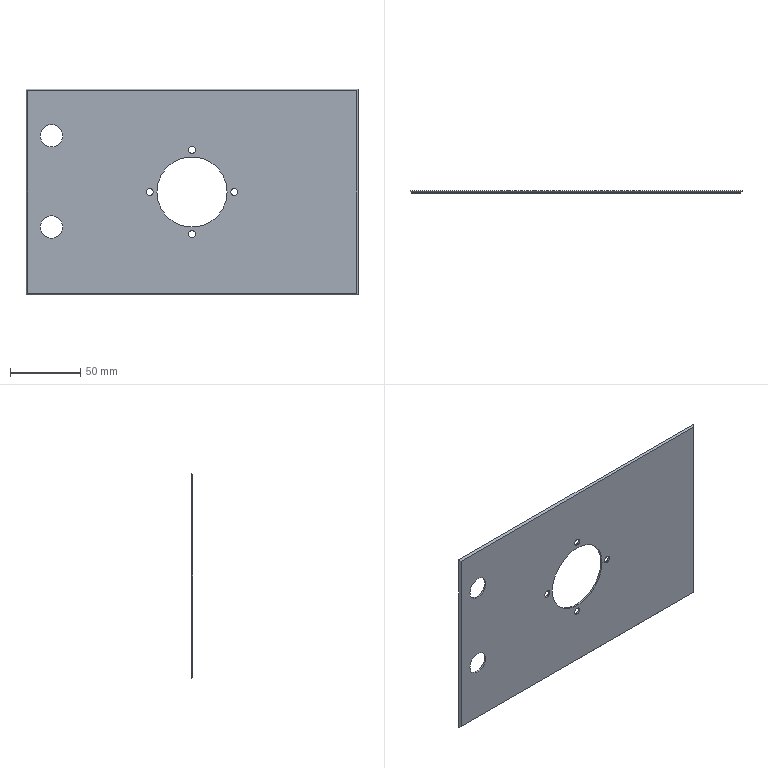Part | NX | 1 solid | 20 faces | box 236.4 x 1.2 x 146.4 mm | volume 38049 mm3 | cylinder 14 | plane 6 | commonest cylinder face diameters 5 x8 16 x4 50 x2
STEP:
#1=CARTESIAN_POINT('',(118.2,-108.8,73.2));
#2=VERTEX_POINT('',#1);
#3=CARTESIAN_POINT('',(118.2,-108.8,-73.2));
#4=VERTEX_POINT('',#3);
#5=CARTESIAN_POINT('',(118.2,-108.8,0.));
#6=DIRECTION('',(0.,0.,-1.));
#7=VECTOR('',#6,1000.);
#8=LINE('',#5,#7);
#9=EDGE_CURVE('',#2,#4,#8,.T.);
#10=ORIENTED_EDGE('',*,*,#9,.T.);
#11=CARTESIAN_POINT('',(-118.2,-108.8,-73.2));
#12=VERTEX_POINT('',#11);
#13=CARTESIAN_POINT('',(0.,-108.8,-73.2));
#14=DIRECTION('',(-1.,0.,0.));
#15=VECTOR('',#14,1000.);
#16=LINE('',#13,#15);
#17=EDGE_CURVE('',#4,#12,#16,.T.);
#18=ORIENTED_EDGE('',*,*,#17,.T.);
#19=CARTESIAN_POINT('',(-118.2,-108.8,73.2));
#20=VERTEX_POINT('',#19);
#21=CARTESIAN_POINT('',(-118.2,-108.8,0.));
#22=DIRECTION('',(0.,0.,-1.));
#23=VECTOR('',#22,1000.);
#24=LINE('',#21,#23);
#25=EDGE_CURVE('',#20,#12,#24,.T.);
#26=ORIENTED_EDGE('',*,*,#25,.F.);
#27=CARTESIAN_POINT('',(0.,-108.8,73.2));
#28=DIRECTION('',(-1.,0.,0.));
#29=VECTOR('',#28,1000.);
#30=LINE('',#27,#29);
#31=EDGE_CURVE('',#2,#20,#30,.T.);
#32=ORIENTED_EDGE('',*,*,#31,.F.);
#33=EDGE_LOOP('',(#10,#18,#26,#32));
#34=FACE_BOUND('',#33,.T.);
#35=CARTESIAN_POINT('',(-2.5,-108.8,-30.));
#36=VERTEX_POINT('',#35);
#37=CARTESIAN_POINT('',(2.5,-108.8,-30.));
#38=VERTEX_POINT('',#37);
#39=CARTESIAN_POINT('',(0.,-108.8,-30.));
#40=DIRECTION('',(0.,1.,0.));
#41=DIRECTION('',(1.,0.,0.));
#42=AXIS2_PLACEMENT_3D('',#39,#40,#41);
#43=CIRCLE('',#42,2.5);
#44=EDGE_CURVE('',#36,#38,#43,.T.);
#45=ORIENTED_EDGE('',*,*,#44,.F.);
#46=CARTESIAN_POINT('',(0.,-108.8,-30.));
#47=DIRECTION('',(0.,1.,0.));
#48=DIRECTION('',(1.,0.,0.));
#49=AXIS2_PLACEMENT_3D('',#46,#47,#48);
#50=CIRCLE('',#49,2.5);
#51=EDGE_CURVE('',#38,#36,#50,.T.);
#52=ORIENTED_EDGE('',*,*,#51,.F.);
#53=EDGE_LOOP('',(#45,#52));
#54=FACE_BOUND('',#53,.T.);
#55=CARTESIAN_POINT('',(32.5,-108.8,0.));
#56=VERTEX_POINT('',#55);
#57=CARTESIAN_POINT('',(27.5,-108.8,0.));
#58=VERTEX_POINT('',#57);
#59=CARTESIAN_POINT('',(30.,-108.8,0.));
#60=DIRECTION('',(0.,1.,0.));
#61=DIRECTION('',(1.,0.,0.));
#62=AXIS2_PLACEMENT_3D('',#59,#60,#61);
#63=CIRCLE('',#62,2.5);
#64=EDGE_CURVE('',#56,#58,#63,.T.);
#65=ORIENTED_EDGE('',*,*,#64,.F.);
#66=CARTESIAN_POINT('',(30.,-108.8,0.));
#67=DIRECTION('',(0.,1.,0.));
#68=DIRECTION('',(1.,0.,0.));
#69=AXIS2_PLACEMENT_3D('',#66,#67,#68);
#70=CIRCLE('',#69,2.5);
#71=EDGE_CURVE('',#58,#56,#70,.T.);
#72=ORIENTED_EDGE('',*,*,#71,.F.);
#73=EDGE_LOOP('',(#65,#72));
#74=FACE_BOUND('',#73,.T.);
#75=CARTESIAN_POINT('',(2.5,-108.8,30.));
#76=VERTEX_POINT('',#75);
#77=CARTESIAN_POINT('',(-2.5,-108.8,30.));
#78=VERTEX_POINT('',#77);
#79=CARTESIAN_POINT('',(0.,-108.8,30.));
#80=DIRECTION('',(0.,1.,0.));
#81=DIRECTION('',(1.,0.,0.));
#82=AXIS2_PLACEMENT_3D('',#79,#80,#81);
#83=CIRCLE('',#82,2.5);
#84=EDGE_CURVE('',#76,#78,#83,.T.);
#85=ORIENTED_EDGE('',*,*,#84,.F.);
#86=CARTESIAN_POINT('',(0.,-108.8,30.));
#87=DIRECTION('',(0.,1.,0.));
#88=DIRECTION('',(1.,0.,0.));
#89=AXIS2_PLACEMENT_3D('',#86,#87,#88);
#90=CIRCLE('',#89,2.5);
#91=EDGE_CURVE('',#78,#76,#90,.T.);
#92=ORIENTED_EDGE('',*,*,#91,.F.);
#93=EDGE_LOOP('',(#85,#92));
#94=FACE_BOUND('',#93,.T.);
#95=CARTESIAN_POINT('',(-32.5,-108.8,0.));
#96=VERTEX_POINT('',#95);
#97=CARTESIAN_POINT('',(-27.5,-108.8,0.));
#98=VERTEX_POINT('',#97);
#99=CARTESIAN_POINT('',(-30.,-108.8,0.));
#100=DIRECTION('',(0.,1.,0.));
#101=DIRECTION('',(1.,0.,0.));
#102=AXIS2_PLACEMENT_3D('',#99,#100,#101);
#103=CIRCLE('',#102,2.5);
#104=EDGE_CURVE('',#96,#98,#103,.T.);
#105=ORIENTED_EDGE('',*,*,#104,.F.);
#106=CARTESIAN_POINT('',(-30.,-108.8,0.));
#107=DIRECTION('',(0.,1.,0.));
#108=DIRECTION('',(1.,0.,0.));
#109=AXIS2_PLACEMENT_3D('',#106,#107,#108);
#110=CIRCLE('',#109,2.5);
#111=EDGE_CURVE('',#98,#96,#110,.T.);
#112=ORIENTED_EDGE('',*,*,#111,.F.);
#113=EDGE_LOOP('',(#105,#112));
#114=FACE_BOUND('',#113,.T.);
#115=CARTESIAN_POINT('',(-108.,-108.8,40.));
#116=VERTEX_POINT('',#115);
#117=CARTESIAN_POINT('',(-92.,-108.8,40.));
#118=VERTEX_POINT('',#117);
#119=CARTESIAN_POINT('',(-100.,-108.8,40.));
#120=DIRECTION('',(0.,-1.,0.));
#121=DIRECTION('',(1.,0.,0.));
#122=AXIS2_PLACEMENT_3D('',#119,#120,#121);
#123=CIRCLE('',#122,8.);
#124=EDGE_CURVE('',#116,#118,#123,.T.);
#125=ORIENTED_EDGE('',*,*,#124,.T.);
#126=CARTESIAN_POINT('',(-100.,-108.8,40.));
#127=DIRECTION('',(0.,-1.,0.));
#128=DIRECTION('',(1.,0.,0.));
#129=AXIS2_PLACEMENT_3D('',#126,#127,#128);
#130=CIRCLE('',#129,8.);
#131=EDGE_CURVE('',#118,#116,#130,.T.);
#132=ORIENTED_EDGE('',*,*,#131,.T.);
#133=EDGE_LOOP('',(#125,#132));
#134=FACE_BOUND('',#133,.T.);
#135=CARTESIAN_POINT('',(-108.,-108.8,-25.));
#136=VERTEX_POINT('',#135);
#137=CARTESIAN_POINT('',(-92.,-108.8,-25.));
#138=VERTEX_POINT('',#137);
#139=CARTESIAN_POINT('',(-100.,-108.8,-25.));
#140=DIRECTION('',(0.,1.,0.));
#141=DIRECTION('',(1.,0.,0.));
#142=AXIS2_PLACEMENT_3D('',#139,#140,#141);
#143=CIRCLE('',#142,8.);
#144=EDGE_CURVE('',#136,#138,#143,.T.);
#145=ORIENTED_EDGE('',*,*,#144,.F.);
#146=CARTESIAN_POINT('',(-100.,-108.8,-25.));
#147=DIRECTION('',(0.,1.,0.));
#148=DIRECTION('',(1.,0.,0.));
#149=AXIS2_PLACEMENT_3D('',#146,#147,#148);
#150=CIRCLE('',#149,8.);
#151=EDGE_CURVE('',#138,#136,#150,.T.);
#152=ORIENTED_EDGE('',*,*,#151,.F.);
#153=EDGE_LOOP('',(#145,#152));
#154=FACE_BOUND('',#153,.T.);
#155=CARTESIAN_POINT('',(25.,-108.8,0.));
#156=VERTEX_POINT('',#155);
#157=CARTESIAN_POINT('',(-25.,-108.8,0.));
#158=VERTEX_POINT('',#157);
#159=CARTESIAN_POINT('',(0.,-108.8,0.));
#160=DIRECTION('',(0.,1.,0.));
#161=DIRECTION('',(1.,0.,0.));
#162=AXIS2_PLACEMENT_3D('',#159,#160,#161);
#163=CIRCLE('',#162,25.);
#164=EDGE_CURVE('',#156,#158,#163,.T.);
#165=ORIENTED_EDGE('',*,*,#164,.F.);
#166=CARTESIAN_POINT('',(0.,-108.8,0.));
#167=DIRECTION('',(0.,1.,0.));
#168=DIRECTION('',(1.,0.,0.));
#169=AXIS2_PLACEMENT_3D('',#166,#167,#168);
#170=CIRCLE('',#169,25.);
#171=EDGE_CURVE('',#158,#156,#170,.T.);
#172=ORIENTED_EDGE('',*,*,#171,.F.);
#173=EDGE_LOOP('',(#165,#172));
#174=FACE_BOUND('',#173,.T.);
#175=CARTESIAN_POINT('',(-120.,-108.8,-75.));
#176=DIRECTION('',(0.,-1.,0.));
#177=DIRECTION('',(0.,0.,-1.));
#178=AXIS2_PLACEMENT_3D('',#175,#176,#177);
#179=PLANE('',#178);
#180=ADVANCED_FACE('',(#34,#54,#74,#94,#114,#134,#154,#174),#179,.F.);
#181=CARTESIAN_POINT('',(117.,-110.,72.));
#182=VERTEX_POINT('',#181);
#183=CARTESIAN_POINT('',(117.,-110.,-72.));
#184=VERTEX_POINT('',#183);
#185=CARTESIAN_POINT('',(117.,-110.,0.));
#186=DIRECTION('',(0.,0.,-1.));
#187=VECTOR('',#186,1000.);
#188=LINE('',#185,#187);
#189=EDGE_CURVE('',#182,#184,#188,.T.);
#190=ORIENTED_EDGE('',*,*,#189,.T.);
#191=CARTESIAN_POINT('',(45.,-182.,0.));
#192=DIRECTION('',(-0.5774,-0.5774,0.5774));
#193=VECTOR('',#192,1000.);
#194=LINE('',#191,#193);
#195=EDGE_CURVE('',#4,#184,#194,.T.);
#196=ORIENTED_EDGE('',*,*,#195,.F.);
#197=ORIENTED_EDGE('',*,*,#9,.F.);
#198=CARTESIAN_POINT('',(45.,-182.,0.));
#199=DIRECTION('',(-0.5774,-0.5774,-0.5774));
#200=VECTOR('',#199,1000.);
#201=LINE('',#198,#200);
#202=EDGE_CURVE('',#2,#182,#201,.T.);
#203=ORIENTED_EDGE('',*,*,#202,.T.);
#204=EDGE_LOOP('',(#190,#196,#197,#203));
#205=FACE_BOUND('',#204,.T.);
#206=CARTESIAN_POINT('',(118.5,-108.5,0.));
#207=DIRECTION('',(-0.7071,0.7071,0.));
#208=DIRECTION('',(0.,0.,1.));
#209=AXIS2_PLACEMENT_3D('',#206,#207,#208);
#210=PLANE('',#209);
#211=ADVANCED_FACE('',(#205),#210,.F.);
#212=CARTESIAN_POINT('',(-117.,-110.,72.));
#213=VERTEX_POINT('',#212);
#214=CARTESIAN_POINT('',(0.,-110.,72.));
#215=DIRECTION('',(-1.,0.,0.));
#216=VECTOR('',#215,1000.);
#217=LINE('',#214,#216);
#218=EDGE_CURVE('',#182,#213,#217,.T.);
#219=ORIENTED_EDGE('',*,*,#218,.F.);
#220=ORIENTED_EDGE('',*,*,#202,.F.);
#221=ORIENTED_EDGE('',*,*,#31,.T.);
#222=CARTESIAN_POINT('',(-45.,-182.,0.));
#223=DIRECTION('',(0.5774,-0.5774,-0.5774));
#224=VECTOR('',#223,1000.);
#225=LINE('',#222,#224);
#226=EDGE_CURVE('',#20,#213,#225,.T.);
#227=ORIENTED_EDGE('',*,*,#226,.T.);
#228=EDGE_LOOP('',(#219,#220,#221,#227));
#229=FACE_BOUND('',#228,.T.);
#230=CARTESIAN_POINT('',(0.,-108.5,73.5));
#231=DIRECTION('',(0.,-0.7071,0.7071));
#232=DIRECTION('',(-1.,0.,0.));
#233=AXIS2_PLACEMENT_3D('',#230,#231,#232);
#234=PLANE('',#233);
#235=ADVANCED_FACE('',(#229),#234,.T.);
#236=CARTESIAN_POINT('',(-117.,-110.,-72.));
#237=VERTEX_POINT('',#236);
#238=CARTESIAN_POINT('',(-117.,-110.,0.));
#239=DIRECTION('',(0.,0.,-1.));
#240=VECTOR('',#239,1000.);
#241=LINE('',#238,#240);
#242=EDGE_CURVE('',#213,#237,#241,.T.);
#243=ORIENTED_EDGE('',*,*,#242,.F.);
#244=ORIENTED_EDGE('',*,*,#226,.F.);
#245=ORIENTED_EDGE('',*,*,#25,.T.);
#246=CARTESIAN_POINT('',(-45.,-182.,0.));
#247=DIRECTION('',(0.5774,-0.5774,0.5774));
#248=VECTOR('',#247,1000.);
#249=LINE('',#246,#248);
#250=EDGE_CURVE('',#12,#237,#249,.T.);
#251=ORIENTED_EDGE('',*,*,#250,.T.);
#252=EDGE_LOOP('',(#243,#244,#245,#251));
#253=FACE_BOUND('',#252,.T.);
#254=CARTESIAN_POINT('',(-118.5,-108.5,0.));
#255=DIRECTION('',(-0.7071,-0.7071,0.));
#256=DIRECTION('',(-0.7071,0.7071,0.));
#257=AXIS2_PLACEMENT_3D('',#254,#255,#256);
#258=PLANE('',#257);
#259=ADVANCED_FACE('',(#253),#258,.T.);
#260=CARTESIAN_POINT('',(0.,-110.,-72.));
#261=DIRECTION('',(-1.,0.,0.));
#262=VECTOR('',#261,1000.);
#263=LINE('',#260,#262);
#264=EDGE_CURVE('',#184,#237,#263,.T.);
#265=ORIENTED_EDGE('',*,*,#264,.T.);
#266=ORIENTED_EDGE('',*,*,#250,.F.);
#267=ORIENTED_EDGE('',*,*,#17,.F.);
#268=ORIENTED_EDGE('',*,*,#195,.T.);
#269=EDGE_LOOP('',(#265,#266,#267,#268));
#270=FACE_BOUND('',#269,.T.);
#271=CARTESIAN_POINT('',(0.,-108.5,-73.5));
#272=DIRECTION('',(0.,0.7071,0.7071));
#273=DIRECTION('',(1.,0.,0.));
#274=AXIS2_PLACEMENT_3D('',#271,#272,#273);
#275=PLANE('',#274);
#276=ADVANCED_FACE('',(#270),#275,.F.);
#277=ORIENTED_EDGE('',*,*,#242,.T.);
#278=ORIENTED_EDGE('',*,*,#264,.F.);
#279=ORIENTED_EDGE('',*,*,#189,.F.);
#280=ORIENTED_EDGE('',*,*,#218,.T.);
#281=EDGE_LOOP('',(#277,#278,#279,#280));
#282=FACE_BOUND('',#281,.T.);
#283=CARTESIAN_POINT('',(27.5,-110.,0.));
#284=VERTEX_POINT('',#283);
#285=CARTESIAN_POINT('',(32.5,-110.,0.));
#286=VERTEX_POINT('',#285);
#287=CARTESIAN_POINT('',(30.,-110.,0.));
#288=DIRECTION('',(0.,-1.,0.));
#289=DIRECTION('',(-1.,0.,0.));
#290=AXIS2_PLACEMENT_3D('',#287,#288,#289);
#291=CIRCLE('',#290,2.5);
#292=EDGE_CURVE('',#284,#286,#291,.T.);
#293=ORIENTED_EDGE('',*,*,#292,.F.);
#294=CARTESIAN_POINT('',(30.,-110.,0.));
#295=DIRECTION('',(0.,-1.,0.));
#296=DIRECTION('',(-1.,0.,0.));
#297=AXIS2_PLACEMENT_3D('',#294,#295,#296);
#298=CIRCLE('',#297,2.5);
#299=EDGE_CURVE('',#286,#284,#298,.T.);
#300=ORIENTED_EDGE('',*,*,#299,.F.);
#301=EDGE_LOOP('',(#293,#300));
#302=FACE_BOUND('',#301,.T.);
#303=CARTESIAN_POINT('',(-2.5,-110.,30.));
#304=VERTEX_POINT('',#303);
#305=CARTESIAN_POINT('',(2.5,-110.,30.));
#306=VERTEX_POINT('',#305);
#307=CARTESIAN_POINT('',(0.,-110.,30.));
#308=DIRECTION('',(0.,-1.,0.));
#309=DIRECTION('',(-1.,0.,0.));
#310=AXIS2_PLACEMENT_3D('',#307,#308,#309);
#311=CIRCLE('',#310,2.5);
#312=EDGE_CURVE('',#304,#306,#311,.T.);
#313=ORIENTED_EDGE('',*,*,#312,.F.);
#314=CARTESIAN_POINT('',(0.,-110.,30.));
#315=DIRECTION('',(0.,-1.,0.));
#316=DIRECTION('',(-1.,0.,0.));
#317=AXIS2_PLACEMENT_3D('',#314,#315,#316);
#318=CIRCLE('',#317,2.5);
#319=EDGE_CURVE('',#306,#304,#318,.T.);
#320=ORIENTED_EDGE('',*,*,#319,.F.);
#321=EDGE_LOOP('',(#313,#320));
#322=FACE_BOUND('',#321,.T.);
#323=CARTESIAN_POINT('',(-32.5,-110.,0.));
#324=VERTEX_POINT('',#323);
#325=CARTESIAN_POINT('',(-27.5,-110.,0.));
#326=VERTEX_POINT('',#325);
#327=CARTESIAN_POINT('',(-30.,-110.,0.));
#328=DIRECTION('',(0.,-1.,0.));
#329=DIRECTION('',(-1.,0.,0.));
#330=AXIS2_PLACEMENT_3D('',#327,#328,#329);
#331=CIRCLE('',#330,2.5);
#332=EDGE_CURVE('',#324,#326,#331,.T.);
#333=ORIENTED_EDGE('',*,*,#332,.F.);
#334=CARTESIAN_POINT('',(-30.,-110.,0.));
#335=DIRECTION('',(0.,-1.,0.));
#336=DIRECTION('',(-1.,0.,0.));
#337=AXIS2_PLACEMENT_3D('',#334,#335,#336);
#338=CIRCLE('',#337,2.5);
#339=EDGE_CURVE('',#326,#324,#338,.T.);
#340=ORIENTED_EDGE('',*,*,#339,.F.);
#341=EDGE_LOOP('',(#333,#340));
#342=FACE_BOUND('',#341,.T.);
#343=CARTESIAN_POINT('',(-108.,-110.,40.));
#344=VERTEX_POINT('',#343);
#345=CARTESIAN_POINT('',(-92.,-110.,40.));
#346=VERTEX_POINT('',#345);
#347=CARTESIAN_POINT('',(-100.,-110.,40.));
#348=DIRECTION('',(0.,-1.,0.));
#349=DIRECTION('',(1.,0.,0.));
#350=AXIS2_PLACEMENT_3D('',#347,#348,#349);
#351=CIRCLE('',#350,8.);
#352=EDGE_CURVE('',#344,#346,#351,.T.);
#353=ORIENTED_EDGE('',*,*,#352,.F.);
#354=CARTESIAN_POINT('',(-100.,-110.,40.));
#355=DIRECTION('',(0.,-1.,0.));
#356=DIRECTION('',(1.,0.,0.));
#357=AXIS2_PLACEMENT_3D('',#354,#355,#356);
#358=CIRCLE('',#357,8.);
#359=EDGE_CURVE('',#346,#344,#358,.T.);
#360=ORIENTED_EDGE('',*,*,#359,.F.);
#361=EDGE_LOOP('',(#353,#360));
#362=FACE_BOUND('',#361,.T.);
#363=CARTESIAN_POINT('',(-108.,-110.,-25.));
#364=VERTEX_POINT('',#363);
#365=CARTESIAN_POINT('',(-92.,-110.,-25.));
#366=VERTEX_POINT('',#365);
#367=CARTESIAN_POINT('',(-100.,-110.,-25.));
#368=DIRECTION('',(0.,-1.,0.));
#369=DIRECTION('',(-1.,0.,0.));
#370=AXIS2_PLACEMENT_3D('',#367,#368,#369);
#371=CIRCLE('',#370,8.);
#372=EDGE_CURVE('',#364,#366,#371,.T.);
#373=ORIENTED_EDGE('',*,*,#372,.F.);
#374=CARTESIAN_POINT('',(-100.,-110.,-25.));
#375=DIRECTION('',(0.,-1.,0.));
#376=DIRECTION('',(-1.,0.,0.));
#377=AXIS2_PLACEMENT_3D('',#374,#375,#376);
#378=CIRCLE('',#377,8.);
#379=EDGE_CURVE('',#366,#364,#378,.T.);
#380=ORIENTED_EDGE('',*,*,#379,.F.);
#381=EDGE_LOOP('',(#373,#380));
#382=FACE_BOUND('',#381,.T.);
#383=CARTESIAN_POINT('',(25.,-110.,0.));
#384=VERTEX_POINT('',#383);
#385=CARTESIAN_POINT('',(-25.,-110.,0.));
#386=VERTEX_POINT('',#385);
#387=CARTESIAN_POINT('',(0.,-110.,0.));
#388=DIRECTION('',(0.,-1.,0.));
#389=DIRECTION('',(-1.,0.,0.));
#390=AXIS2_PLACEMENT_3D('',#387,#388,#389);
#391=CIRCLE('',#390,25.);
#392=EDGE_CURVE('',#384,#386,#391,.T.);
#393=ORIENTED_EDGE('',*,*,#392,.F.);
#394=CARTESIAN_POINT('',(0.,-110.,0.));
#395=DIRECTION('',(0.,-1.,0.));
#396=DIRECTION('',(-1.,0.,0.));
#397=AXIS2_PLACEMENT_3D('',#394,#395,#396);
#398=CIRCLE('',#397,25.);
#399=EDGE_CURVE('',#386,#384,#398,.T.);
#400=ORIENTED_EDGE('',*,*,#399,.F.);
#401=EDGE_LOOP('',(#393,#400));
#402=FACE_BOUND('',#401,.T.);
#403=CARTESIAN_POINT('',(-2.5,-110.,-30.));
#404=VERTEX_POINT('',#403);
#405=CARTESIAN_POINT('',(2.5,-110.,-30.));
#406=VERTEX_POINT('',#405);
#407=CARTESIAN_POINT('',(0.,-110.,-30.));
#408=DIRECTION('',(0.,-1.,0.));
#409=DIRECTION('',(-1.,0.,0.));
#410=AXIS2_PLACEMENT_3D('',#407,#408,#409);
#411=CIRCLE('',#410,2.5);
#412=EDGE_CURVE('',#404,#406,#411,.T.);
#413=ORIENTED_EDGE('',*,*,#412,.F.);
#414=CARTESIAN_POINT('',(0.,-110.,-30.));
#415=DIRECTION('',(0.,-1.,0.));
#416=DIRECTION('',(-1.,0.,0.));
#417=AXIS2_PLACEMENT_3D('',#414,#415,#416);
#418=CIRCLE('',#417,2.5);
#419=EDGE_CURVE('',#406,#404,#418,.T.);
#420=ORIENTED_EDGE('',*,*,#419,.F.);
#421=EDGE_LOOP('',(#413,#420));
#422=FACE_BOUND('',#421,.T.);
#423=CARTESIAN_POINT('',(-120.,-110.,-75.));
#424=DIRECTION('',(0.,-1.,0.));
#425=DIRECTION('',(0.,0.,-1.));
#426=AXIS2_PLACEMENT_3D('',#423,#424,#425);
#427=PLANE('',#426);
#428=ADVANCED_FACE('',(#282,#302,#322,#342,#362,#382,#402,#422),#427,.T.);
#429=ORIENTED_EDGE('',*,*,#292,.T.);
#430=CARTESIAN_POINT('',(32.5,-110.,0.));
#431=DIRECTION('',(0.,1.,0.));
#432=VECTOR('',#431,1000.);
#433=LINE('',#430,#432);
#434=EDGE_CURVE('',#56,#286,#433,.F.);
#435=ORIENTED_EDGE('',*,*,#434,.F.);
#436=ORIENTED_EDGE('',*,*,#64,.T.);
#437=CARTESIAN_POINT('',(27.5,-110.,0.));
#438=DIRECTION('',(0.,1.,0.));
#439=VECTOR('',#438,1000.);
#440=LINE('',#437,#439);
#441=EDGE_CURVE('',#58,#284,#440,.F.);
#442=ORIENTED_EDGE('',*,*,#441,.T.);
#443=EDGE_LOOP('',(#429,#435,#436,#442));
#444=FACE_BOUND('',#443,.T.);
#445=CARTESIAN_POINT('',(30.,-110.,0.));
#446=DIRECTION('',(0.,1.,0.));
#447=DIRECTION('',(-1.,0.,0.));
#448=AXIS2_PLACEMENT_3D('',#445,#446,#447);
#449=CYLINDRICAL_SURFACE('',#448,2.5);
#450=ADVANCED_FACE('',(#444),#449,.F.);
#451=ORIENTED_EDGE('',*,*,#312,.T.);
#452=CARTESIAN_POINT('',(2.5,-110.,30.));
#453=DIRECTION('',(0.,1.,0.));
#454=VECTOR('',#453,1000.);
#455=LINE('',#452,#454);
#456=EDGE_CURVE('',#76,#306,#455,.F.);
#457=ORIENTED_EDGE('',*,*,#456,.F.);
#458=ORIENTED_EDGE('',*,*,#84,.T.);
#459=CARTESIAN_POINT('',(-2.5,-110.,30.));
#460=DIRECTION('',(0.,1.,0.));
#461=VECTOR('',#460,1000.);
#462=LINE('',#459,#461);
#463=EDGE_CURVE('',#78,#304,#462,.F.);
#464=ORIENTED_EDGE('',*,*,#463,.T.);
#465=EDGE_LOOP('',(#451,#457,#458,#464));
#466=FACE_BOUND('',#465,.T.);
#467=CARTESIAN_POINT('',(0.,-110.,30.));
#468=DIRECTION('',(0.,1.,0.));
#469=DIRECTION('',(-1.,0.,0.));
#470=AXIS2_PLACEMENT_3D('',#467,#468,#469);
#471=CYLINDRICAL_SURFACE('',#470,2.5);
#472=ADVANCED_FACE('',(#466),#471,.F.);
#473=ORIENTED_EDGE('',*,*,#104,.T.);
#474=CARTESIAN_POINT('',(-27.5,-110.,0.));
#475=DIRECTION('',(0.,1.,0.));
#476=VECTOR('',#475,1000.);
#477=LINE('',#474,#476);
#478=EDGE_CURVE('',#326,#98,#477,.T.);
#479=ORIENTED_EDGE('',*,*,#478,.F.);
#480=ORIENTED_EDGE('',*,*,#339,.T.);
#481=CARTESIAN_POINT('',(-32.5,-110.,0.));
#482=DIRECTION('',(0.,1.,0.));
#483=VECTOR('',#482,1000.);
#484=LINE('',#481,#483);
#485=EDGE_CURVE('',#324,#96,#484,.T.);
#486=ORIENTED_EDGE('',*,*,#485,.T.);
#487=EDGE_LOOP('',(#473,#479,#480,#486));
#488=FACE_BOUND('',#487,.T.);
#489=CARTESIAN_POINT('',(-30.,-110.,0.));
#490=DIRECTION('',(0.,1.,0.));
#491=DIRECTION('',(-1.,0.,0.));
#492=AXIS2_PLACEMENT_3D('',#489,#490,#491);
#493=CYLINDRICAL_SURFACE('',#492,2.5);
#494=ADVANCED_FACE('',(#488),#493,.F.);
#495=ORIENTED_EDGE('',*,*,#352,.T.);
#496=CARTESIAN_POINT('',(-92.,-110.,40.));
#497=DIRECTION('',(0.,-1.,0.));
#498=VECTOR('',#497,1000.);
#499=LINE('',#496,#498);
#500=EDGE_CURVE('',#118,#346,#499,.T.);
#501=ORIENTED_EDGE('',*,*,#500,.F.);
#502=ORIENTED_EDGE('',*,*,#124,.F.);
#503=CARTESIAN_POINT('',(-108.,-110.,40.));
#504=DIRECTION('',(0.,-1.,0.));
#505=VECTOR('',#504,1000.);
#506=LINE('',#503,#505);
#507=EDGE_CURVE('',#116,#344,#506,.T.);
#508=ORIENTED_EDGE('',*,*,#507,.T.);
#509=EDGE_LOOP('',(#495,#501,#502,#508));
#510=FACE_BOUND('',#509,.T.);
#511=CARTESIAN_POINT('',(-100.,-110.,40.));
#512=DIRECTION('',(0.,-1.,0.));
#513=DIRECTION('',(1.,0.,0.));
#514=AXIS2_PLACEMENT_3D('',#511,#512,#513);
#515=CYLINDRICAL_SURFACE('',#514,8.);
#516=ADVANCED_FACE('',(#510),#515,.F.);
#517=ORIENTED_EDGE('',*,*,#144,.T.);
#518=CARTESIAN_POINT('',(-92.,-110.,-25.));
#519=DIRECTION('',(0.,1.,0.));
#520=VECTOR('',#519,1000.);
#521=LINE('',#518,#520);
#522=EDGE_CURVE('',#366,#138,#521,.T.);
#523=ORIENTED_EDGE('',*,*,#522,.F.);
#524=ORIENTED_EDGE('',*,*,#379,.T.);
#525=CARTESIAN_POINT('',(-108.,-110.,-25.));
#526=DIRECTION('',(0.,1.,0.));
#527=VECTOR('',#526,1000.);
#528=LINE('',#525,#527);
#529=EDGE_CURVE('',#364,#136,#528,.T.);
#530=ORIENTED_EDGE('',*,*,#529,.T.);
#531=EDGE_LOOP('',(#517,#523,#524,#530));
#532=FACE_BOUND('',#531,.T.);
#533=CARTESIAN_POINT('',(-100.,-110.,-25.));
#534=DIRECTION('',(0.,1.,0.));
#535=DIRECTION('',(-1.,0.,0.));
#536=AXIS2_PLACEMENT_3D('',#533,#534,#535);
#537=CYLINDRICAL_SURFACE('',#536,8.);
#538=ADVANCED_FACE('',(#532),#537,.F.);
#539=ORIENTED_EDGE('',*,*,#392,.T.);
#540=CARTESIAN_POINT('',(-25.,-110.,0.));
#541=DIRECTION('',(0.,1.,0.));
#542=VECTOR('',#541,1000.);
#543=LINE('',#540,#542);
#544=EDGE_CURVE('',#158,#386,#543,.F.);
#545=ORIENTED_EDGE('',*,*,#544,.F.);
#546=ORIENTED_EDGE('',*,*,#171,.T.);
#547=CARTESIAN_POINT('',(25.,-110.,0.));
#548=DIRECTION('',(0.,1.,0.));
#549=VECTOR('',#548,1000.);
#550=LINE('',#547,#549);
#551=EDGE_CURVE('',#156,#384,#550,.F.);
#552=ORIENTED_EDGE('',*,*,#551,.T.);
#553=EDGE_LOOP('',(#539,#545,#546,#552));
#554=FACE_BOUND('',#553,.T.);
#555=CARTESIAN_POINT('',(0.,-110.,0.));
#556=DIRECTION('',(0.,1.,0.));
#557=DIRECTION('',(-1.,0.,0.));
#558=AXIS2_PLACEMENT_3D('',#555,#556,#557);
#559=CYLINDRICAL_SURFACE('',#558,25.);
#560=ADVANCED_FACE('',(#554),#559,.F.);
#561=ORIENTED_EDGE('',*,*,#44,.T.);
#562=CARTESIAN_POINT('',(2.5,-110.,-30.));
#563=DIRECTION('',(0.,1.,0.));
#564=VECTOR('',#563,1000.);
#565=LINE('',#562,#564);
#566=EDGE_CURVE('',#406,#38,#565,.T.);
#567=ORIENTED_EDGE('',*,*,#566,.F.);
#568=ORIENTED_EDGE('',*,*,#419,.T.);
#569=CARTESIAN_POINT('',(-2.5,-110.,-30.));
#570=DIRECTION('',(0.,1.,0.));
#571=VECTOR('',#570,1000.);
#572=LINE('',#569,#571);
#573=EDGE_CURVE('',#404,#36,#572,.T.);
#574=ORIENTED_EDGE('',*,*,#573,.T.);
#575=EDGE_LOOP('',(#561,#567,#568,#574));
#576=FACE_BOUND('',#575,.T.);
#577=CARTESIAN_POINT('',(0.,-110.,-30.));
#578=DIRECTION('',(0.,1.,0.));
#579=DIRECTION('',(-1.,0.,0.));
#580=AXIS2_PLACEMENT_3D('',#577,#578,#579);
#581=CYLINDRICAL_SURFACE('',#580,2.5);
#582=ADVANCED_FACE('',(#576),#581,.F.);
#583=ORIENTED_EDGE('',*,*,#500,.T.);
#584=ORIENTED_EDGE('',*,*,#359,.T.);
#585=ORIENTED_EDGE('',*,*,#507,.F.);
#586=ORIENTED_EDGE('',*,*,#131,.F.);
#587=EDGE_LOOP('',(#583,#584,#585,#586));
#588=FACE_BOUND('',#587,.T.);
#589=CARTESIAN_POINT('',(-100.,-110.,40.));
#590=DIRECTION('',(0.,-1.,0.));
#591=DIRECTION('',(1.,0.,0.));
#592=AXIS2_PLACEMENT_3D('',#589,#590,#591);
#593=CYLINDRICAL_SURFACE('',#592,8.);
#594=ADVANCED_FACE('',(#588),#593,.F.);
#595=ORIENTED_EDGE('',*,*,#332,.T.);
#596=ORIENTED_EDGE('',*,*,#478,.T.);
#597=ORIENTED_EDGE('',*,*,#111,.T.);
#598=ORIENTED_EDGE('',*,*,#485,.F.);
#599=EDGE_LOOP('',(#595,#596,#597,#598));
#600=FACE_BOUND('',#599,.T.);
#601=CARTESIAN_POINT('',(-30.,-110.,0.));
#602=DIRECTION('',(0.,1.,0.));
#603=DIRECTION('',(-1.,0.,0.));
#604=AXIS2_PLACEMENT_3D('',#601,#602,#603);
#605=CYLINDRICAL_SURFACE('',#604,2.5);
#606=ADVANCED_FACE('',(#600),#605,.F.);
#607=ORIENTED_EDGE('',*,*,#463,.F.);
#608=ORIENTED_EDGE('',*,*,#91,.T.);
#609=ORIENTED_EDGE('',*,*,#456,.T.);
#610=ORIENTED_EDGE('',*,*,#319,.T.);
#611=EDGE_LOOP('',(#607,#608,#609,#610));
#612=FACE_BOUND('',#611,.T.);
#613=CARTESIAN_POINT('',(0.,-110.,30.));
#614=DIRECTION('',(0.,1.,0.));
#615=DIRECTION('',(-1.,0.,0.));
#616=AXIS2_PLACEMENT_3D('',#613,#614,#615);
#617=CYLINDRICAL_SURFACE('',#616,2.5);
#618=ADVANCED_FACE('',(#612),#617,.F.);
#619=ORIENTED_EDGE('',*,*,#441,.F.);
#620=ORIENTED_EDGE('',*,*,#71,.T.);
#621=ORIENTED_EDGE('',*,*,#434,.T.);
#622=ORIENTED_EDGE('',*,*,#299,.T.);
#623=EDGE_LOOP('',(#619,#620,#621,#622));
#624=FACE_BOUND('',#623,.T.);
#625=CARTESIAN_POINT('',(30.,-110.,0.));
#626=DIRECTION('',(0.,1.,0.));
#627=DIRECTION('',(-1.,0.,0.));
#628=AXIS2_PLACEMENT_3D('',#625,#626,#627);
#629=CYLINDRICAL_SURFACE('',#628,2.5);
#630=ADVANCED_FACE('',(#624),#629,.F.);
#631=ORIENTED_EDGE('',*,*,#412,.T.);
#632=ORIENTED_EDGE('',*,*,#566,.T.);
#633=ORIENTED_EDGE('',*,*,#51,.T.);
#634=ORIENTED_EDGE('',*,*,#573,.F.);
#635=EDGE_LOOP('',(#631,#632,#633,#634));
#636=FACE_BOUND('',#635,.T.);
#637=CARTESIAN_POINT('',(0.,-110.,-30.));
#638=DIRECTION('',(0.,1.,0.));
#639=DIRECTION('',(-1.,0.,0.));
#640=AXIS2_PLACEMENT_3D('',#637,#638,#639);
#641=CYLINDRICAL_SURFACE('',#640,2.5);
#642=ADVANCED_FACE('',(#636),#641,.F.);
#643=ORIENTED_EDGE('',*,*,#164,.T.);
#644=ORIENTED_EDGE('',*,*,#544,.T.);
#645=ORIENTED_EDGE('',*,*,#399,.T.);
#646=ORIENTED_EDGE('',*,*,#551,.F.);
#647=EDGE_LOOP('',(#643,#644,#645,#646));
#648=FACE_BOUND('',#647,.T.);
#649=CARTESIAN_POINT('',(0.,-110.,0.));
#650=DIRECTION('',(0.,1.,0.));
#651=DIRECTION('',(-1.,0.,0.));
#652=AXIS2_PLACEMENT_3D('',#649,#650,#651);
#653=CYLINDRICAL_SURFACE('',#652,25.);
#654=ADVANCED_FACE('',(#648),#653,.F.);
#655=ORIENTED_EDGE('',*,*,#372,.T.);
#656=ORIENTED_EDGE('',*,*,#522,.T.);
#657=ORIENTED_EDGE('',*,*,#151,.T.);
#658=ORIENTED_EDGE('',*,*,#529,.F.);
#659=EDGE_LOOP('',(#655,#656,#657,#658));
#660=FACE_BOUND('',#659,.T.);
#661=CARTESIAN_POINT('',(-100.,-110.,-25.));
#662=DIRECTION('',(0.,1.,0.));
#663=DIRECTION('',(-1.,0.,0.));
#664=AXIS2_PLACEMENT_3D('',#661,#662,#663);
#665=CYLINDRICAL_SURFACE('',#664,8.);
#666=ADVANCED_FACE('',(#660),#665,.F.);
#667=CLOSED_SHELL('',(#180,#211,#235,#259,#276,#428,#450,#472,#494,#516,#538,#560,#582,#594,#606,#618,#630,#642,#654,#666));
#668=MANIFOLD_SOLID_BREP('',#667);
#669=(LENGTH_UNIT()NAMED_UNIT(*)SI_UNIT(.MILLI.,.METRE.));
#670=UNCERTAINTY_MEASURE_WITH_UNIT(LENGTH_MEASURE(0.00001),#669,'','');
#671=(NAMED_UNIT(*)PLANE_ANGLE_UNIT()SI_UNIT($,.RADIAN.));
#672=(NAMED_UNIT(*)SI_UNIT($,.STERADIAN.)SOLID_ANGLE_UNIT());
#673=(GEOMETRIC_REPRESENTATION_CONTEXT(3)GLOBAL_UNCERTAINTY_ASSIGNED_CONTEXT((#670))GLOBAL_UNIT_ASSIGNED_CONTEXT((#669,#671,#672))REPRESENTATION_CONTEXT('',''));
#674=ADVANCED_BREP_SHAPE_REPRESENTATION('',(#668),#673);